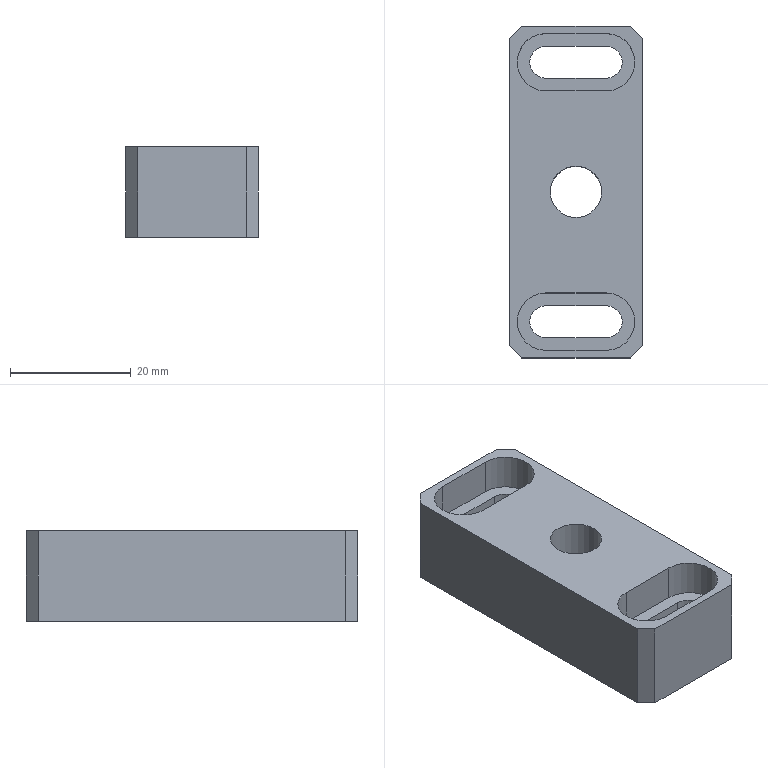Part | NX | 1 solid | 29 faces | box 22 x 55 x 15 mm | volume 13837 mm3 | plane 20 | cylinder 9 | commonest cylinder face diameters 5.3 x4 9.5 x4 8.5 x1
STEP:
#1=CARTESIAN_POINT('',(-5.,16.75,15.));
#2=VERTEX_POINT('',#1);
#3=CARTESIAN_POINT('',(5.,16.75,15.));
#4=VERTEX_POINT('',#3);
#5=CARTESIAN_POINT('',(-5.,16.75,15.));
#6=DIRECTION('',(1.,0.,0.));
#7=VECTOR('',#6,1000.);
#8=LINE('',#5,#7);
#9=EDGE_CURVE('',#2,#4,#8,.T.);
#10=ORIENTED_EDGE('',*,*,#9,.F.);
#11=CARTESIAN_POINT('',(-5.,26.25,15.));
#12=VERTEX_POINT('',#11);
#13=CARTESIAN_POINT('',(-5.,21.5,15.));
#14=DIRECTION('',(0.,0.,1.));
#15=DIRECTION('',(1.,0.,0.));
#16=AXIS2_PLACEMENT_3D('',#13,#14,#15);
#17=CIRCLE('',#16,4.75);
#18=EDGE_CURVE('',#12,#2,#17,.T.);
#19=ORIENTED_EDGE('',*,*,#18,.F.);
#20=CARTESIAN_POINT('',(5.,26.25,15.));
#21=VERTEX_POINT('',#20);
#22=CARTESIAN_POINT('',(-5.,26.25,15.));
#23=DIRECTION('',(-1.,0.,0.));
#24=VECTOR('',#23,1000.);
#25=LINE('',#22,#24);
#26=EDGE_CURVE('',#21,#12,#25,.T.);
#27=ORIENTED_EDGE('',*,*,#26,.F.);
#28=CARTESIAN_POINT('',(5.,21.5,15.));
#29=DIRECTION('',(0.,0.,1.));
#30=DIRECTION('',(1.,0.,0.));
#31=AXIS2_PLACEMENT_3D('',#28,#29,#30);
#32=CIRCLE('',#31,4.75);
#33=EDGE_CURVE('',#4,#21,#32,.T.);
#34=ORIENTED_EDGE('',*,*,#33,.F.);
#35=EDGE_LOOP('',(#10,#19,#27,#34));
#36=FACE_BOUND('',#35,.T.);
#37=CARTESIAN_POINT('',(4.25,0.,15.));
#38=VERTEX_POINT('',#37);
#39=CARTESIAN_POINT('',(0.,0.,15.));
#40=DIRECTION('',(0.,0.,1.));
#41=DIRECTION('',(1.,0.,0.));
#42=AXIS2_PLACEMENT_3D('',#39,#40,#41);
#43=CIRCLE('',#42,4.25);
#44=EDGE_CURVE('',#38,#38,#43,.T.);
#45=ORIENTED_EDGE('',*,*,#44,.F.);
#46=EDGE_LOOP('',(#45));
#47=FACE_BOUND('',#46,.T.);
#48=CARTESIAN_POINT('',(-11.,25.5,15.));
#49=VERTEX_POINT('',#48);
#50=CARTESIAN_POINT('',(-11.,-25.5,15.));
#51=VERTEX_POINT('',#50);
#52=CARTESIAN_POINT('',(-11.,-27.5,15.));
#53=DIRECTION('',(0.,-1.,0.));
#54=VECTOR('',#53,1000.);
#55=LINE('',#52,#54);
#56=EDGE_CURVE('',#49,#51,#55,.T.);
#57=ORIENTED_EDGE('',*,*,#56,.T.);
#58=CARTESIAN_POINT('',(-9.,-27.5,15.));
#59=VERTEX_POINT('',#58);
#60=CARTESIAN_POINT('',(-9.,-27.5,15.));
#61=DIRECTION('',(-0.7071,0.7071,0.));
#62=VECTOR('',#61,1000.);
#63=LINE('',#60,#62);
#64=EDGE_CURVE('',#51,#59,#63,.F.);
#65=ORIENTED_EDGE('',*,*,#64,.T.);
#66=CARTESIAN_POINT('',(9.,-27.5,15.));
#67=VERTEX_POINT('',#66);
#68=CARTESIAN_POINT('',(-11.,-27.5,15.));
#69=DIRECTION('',(1.,0.,0.));
#70=VECTOR('',#69,1000.);
#71=LINE('',#68,#70);
#72=EDGE_CURVE('',#59,#67,#71,.T.);
#73=ORIENTED_EDGE('',*,*,#72,.T.);
#74=CARTESIAN_POINT('',(11.,-25.5,15.));
#75=VERTEX_POINT('',#74);
#76=CARTESIAN_POINT('',(11.,-25.5,15.));
#77=DIRECTION('',(-0.7071,-0.7071,0.));
#78=VECTOR('',#77,1000.);
#79=LINE('',#76,#78);
#80=EDGE_CURVE('',#67,#75,#79,.F.);
#81=ORIENTED_EDGE('',*,*,#80,.T.);
#82=CARTESIAN_POINT('',(11.,25.5,15.));
#83=VERTEX_POINT('',#82);
#84=CARTESIAN_POINT('',(11.,-27.5,15.));
#85=DIRECTION('',(0.,1.,0.));
#86=VECTOR('',#85,1000.);
#87=LINE('',#84,#86);
#88=EDGE_CURVE('',#75,#83,#87,.T.);
#89=ORIENTED_EDGE('',*,*,#88,.T.);
#90=CARTESIAN_POINT('',(9.,27.5,15.));
#91=VERTEX_POINT('',#90);
#92=CARTESIAN_POINT('',(9.,27.5,15.));
#93=DIRECTION('',(0.7071,-0.7071,0.));
#94=VECTOR('',#93,1000.);
#95=LINE('',#92,#94);
#96=EDGE_CURVE('',#83,#91,#95,.F.);
#97=ORIENTED_EDGE('',*,*,#96,.T.);
#98=CARTESIAN_POINT('',(-9.,27.5,15.));
#99=VERTEX_POINT('',#98);
#100=CARTESIAN_POINT('',(-11.,27.5,15.));
#101=DIRECTION('',(-1.,0.,0.));
#102=VECTOR('',#101,1000.);
#103=LINE('',#100,#102);
#104=EDGE_CURVE('',#91,#99,#103,.T.);
#105=ORIENTED_EDGE('',*,*,#104,.T.);
#106=CARTESIAN_POINT('',(-11.,25.5,15.));
#107=DIRECTION('',(0.7071,0.7071,0.));
#108=VECTOR('',#107,1000.);
#109=LINE('',#106,#108);
#110=EDGE_CURVE('',#99,#49,#109,.F.);
#111=ORIENTED_EDGE('',*,*,#110,.T.);
#112=EDGE_LOOP('',(#57,#65,#73,#81,#89,#97,#105,#111));
#113=FACE_BOUND('',#112,.T.);
#114=CARTESIAN_POINT('',(-5.,-26.25,15.));
#115=VERTEX_POINT('',#114);
#116=CARTESIAN_POINT('',(-5.,-16.75,15.));
#117=VERTEX_POINT('',#116);
#118=CARTESIAN_POINT('',(-5.,-21.5,15.));
#119=DIRECTION('',(0.,0.,-1.));
#120=DIRECTION('',(1.,0.,0.));
#121=AXIS2_PLACEMENT_3D('',#118,#119,#120);
#122=CIRCLE('',#121,4.75);
#123=EDGE_CURVE('',#115,#117,#122,.T.);
#124=ORIENTED_EDGE('',*,*,#123,.T.);
#125=CARTESIAN_POINT('',(5.,-16.75,15.));
#126=VERTEX_POINT('',#125);
#127=CARTESIAN_POINT('',(-5.,-16.75,15.));
#128=DIRECTION('',(1.,0.,0.));
#129=VECTOR('',#128,1000.);
#130=LINE('',#127,#129);
#131=EDGE_CURVE('',#117,#126,#130,.T.);
#132=ORIENTED_EDGE('',*,*,#131,.T.);
#133=CARTESIAN_POINT('',(5.,-26.25,15.));
#134=VERTEX_POINT('',#133);
#135=CARTESIAN_POINT('',(5.,-21.5,15.));
#136=DIRECTION('',(0.,0.,-1.));
#137=DIRECTION('',(1.,0.,0.));
#138=AXIS2_PLACEMENT_3D('',#135,#136,#137);
#139=CIRCLE('',#138,4.75);
#140=EDGE_CURVE('',#126,#134,#139,.T.);
#141=ORIENTED_EDGE('',*,*,#140,.T.);
#142=CARTESIAN_POINT('',(-5.,-26.25,15.));
#143=DIRECTION('',(-1.,0.,0.));
#144=VECTOR('',#143,1000.);
#145=LINE('',#142,#144);
#146=EDGE_CURVE('',#134,#115,#145,.T.);
#147=ORIENTED_EDGE('',*,*,#146,.T.);
#148=EDGE_LOOP('',(#124,#132,#141,#147));
#149=FACE_BOUND('',#148,.T.);
#150=CARTESIAN_POINT('',(0.,0.,15.));
#151=DIRECTION('',(0.,0.,-1.));
#152=DIRECTION('',(-1.,0.,0.));
#153=AXIS2_PLACEMENT_3D('',#150,#151,#152);
#154=PLANE('',#153);
#155=ADVANCED_FACE('',(#36,#47,#113,#149),#154,.F.);
#156=CARTESIAN_POINT('',(-5.,-18.85,0.));
#157=VERTEX_POINT('',#156);
#158=CARTESIAN_POINT('',(-5.,-18.85,9.));
#159=VERTEX_POINT('',#158);
#160=CARTESIAN_POINT('',(-5.,-18.85,0.));
#161=DIRECTION('',(0.,0.,1.));
#162=VECTOR('',#161,1000.);
#163=LINE('',#160,#162);
#164=EDGE_CURVE('',#157,#159,#163,.T.);
#165=ORIENTED_EDGE('',*,*,#164,.T.);
#166=CARTESIAN_POINT('',(-5.,-24.15,9.));
#167=VERTEX_POINT('',#166);
#168=CARTESIAN_POINT('',(-5.,-21.5,9.));
#169=DIRECTION('',(0.,0.,1.));
#170=DIRECTION('',(1.,0.,0.));
#171=AXIS2_PLACEMENT_3D('',#168,#169,#170);
#172=CIRCLE('',#171,2.65);
#173=EDGE_CURVE('',#159,#167,#172,.T.);
#174=ORIENTED_EDGE('',*,*,#173,.T.);
#175=CARTESIAN_POINT('',(-5.,-24.15,0.));
#176=VERTEX_POINT('',#175);
#177=CARTESIAN_POINT('',(-5.,-24.15,0.));
#178=DIRECTION('',(0.,0.,1.));
#179=VECTOR('',#178,1000.);
#180=LINE('',#177,#179);
#181=EDGE_CURVE('',#176,#167,#180,.T.);
#182=ORIENTED_EDGE('',*,*,#181,.F.);
#183=CARTESIAN_POINT('',(-5.,-21.5,0.));
#184=DIRECTION('',(0.,0.,-1.));
#185=DIRECTION('',(1.,0.,0.));
#186=AXIS2_PLACEMENT_3D('',#183,#184,#185);
#187=CIRCLE('',#186,2.65);
#188=EDGE_CURVE('',#176,#157,#187,.T.);
#189=ORIENTED_EDGE('',*,*,#188,.T.);
#190=EDGE_LOOP('',(#165,#174,#182,#189));
#191=FACE_BOUND('',#190,.T.);
#192=CARTESIAN_POINT('',(-5.,-21.5,0.));
#193=DIRECTION('',(0.,0.,1.));
#194=DIRECTION('',(1.,0.,0.));
#195=AXIS2_PLACEMENT_3D('',#192,#193,#194);
#196=CYLINDRICAL_SURFACE('',#195,2.65);
#197=ADVANCED_FACE('',(#191),#196,.F.);
#198=CARTESIAN_POINT('',(5.,-18.85,0.));
#199=VERTEX_POINT('',#198);
#200=CARTESIAN_POINT('',(5.,-18.85,9.));
#201=VERTEX_POINT('',#200);
#202=CARTESIAN_POINT('',(5.,-18.85,0.));
#203=DIRECTION('',(0.,0.,1.));
#204=VECTOR('',#203,1000.);
#205=LINE('',#202,#204);
#206=EDGE_CURVE('',#199,#201,#205,.T.);
#207=ORIENTED_EDGE('',*,*,#206,.T.);
#208=CARTESIAN_POINT('',(-5.,-18.85,9.));
#209=DIRECTION('',(-1.,0.,0.));
#210=VECTOR('',#209,1000.);
#211=LINE('',#208,#210);
#212=EDGE_CURVE('',#201,#159,#211,.T.);
#213=ORIENTED_EDGE('',*,*,#212,.T.);
#214=ORIENTED_EDGE('',*,*,#164,.F.);
#215=CARTESIAN_POINT('',(-5.,-18.85,0.));
#216=DIRECTION('',(1.,0.,0.));
#217=VECTOR('',#216,1000.);
#218=LINE('',#215,#217);
#219=EDGE_CURVE('',#157,#199,#218,.T.);
#220=ORIENTED_EDGE('',*,*,#219,.T.);
#221=EDGE_LOOP('',(#207,#213,#214,#220));
#222=FACE_BOUND('',#221,.T.);
#223=CARTESIAN_POINT('',(-5.,-18.85,0.));
#224=DIRECTION('',(0.,-1.,0.));
#225=DIRECTION('',(0.,0.,-1.));
#226=AXIS2_PLACEMENT_3D('',#223,#224,#225);
#227=PLANE('',#226);
#228=ADVANCED_FACE('',(#222),#227,.T.);
#229=CARTESIAN_POINT('',(5.,-24.15,0.));
#230=VERTEX_POINT('',#229);
#231=CARTESIAN_POINT('',(5.,-24.15,9.));
#232=VERTEX_POINT('',#231);
#233=CARTESIAN_POINT('',(5.,-24.15,0.));
#234=DIRECTION('',(0.,0.,1.));
#235=VECTOR('',#234,1000.);
#236=LINE('',#233,#235);
#237=EDGE_CURVE('',#230,#232,#236,.T.);
#238=ORIENTED_EDGE('',*,*,#237,.T.);
#239=CARTESIAN_POINT('',(5.,-21.5,9.));
#240=DIRECTION('',(0.,0.,1.));
#241=DIRECTION('',(1.,0.,0.));
#242=AXIS2_PLACEMENT_3D('',#239,#240,#241);
#243=CIRCLE('',#242,2.65);
#244=EDGE_CURVE('',#232,#201,#243,.T.);
#245=ORIENTED_EDGE('',*,*,#244,.T.);
#246=ORIENTED_EDGE('',*,*,#206,.F.);
#247=CARTESIAN_POINT('',(5.,-21.5,0.));
#248=DIRECTION('',(0.,0.,-1.));
#249=DIRECTION('',(1.,0.,0.));
#250=AXIS2_PLACEMENT_3D('',#247,#248,#249);
#251=CIRCLE('',#250,2.65);
#252=EDGE_CURVE('',#199,#230,#251,.T.);
#253=ORIENTED_EDGE('',*,*,#252,.T.);
#254=EDGE_LOOP('',(#238,#245,#246,#253));
#255=FACE_BOUND('',#254,.T.);
#256=CARTESIAN_POINT('',(5.,-21.5,0.));
#257=DIRECTION('',(0.,0.,1.));
#258=DIRECTION('',(1.,0.,0.));
#259=AXIS2_PLACEMENT_3D('',#256,#257,#258);
#260=CYLINDRICAL_SURFACE('',#259,2.65);
#261=ADVANCED_FACE('',(#255),#260,.F.);
#262=ORIENTED_EDGE('',*,*,#181,.T.);
#263=CARTESIAN_POINT('',(-5.,-24.15,9.));
#264=DIRECTION('',(1.,0.,0.));
#265=VECTOR('',#264,1000.);
#266=LINE('',#263,#265);
#267=EDGE_CURVE('',#167,#232,#266,.T.);
#268=ORIENTED_EDGE('',*,*,#267,.T.);
#269=ORIENTED_EDGE('',*,*,#237,.F.);
#270=CARTESIAN_POINT('',(-5.,-24.15,0.));
#271=DIRECTION('',(-1.,0.,0.));
#272=VECTOR('',#271,1000.);
#273=LINE('',#270,#272);
#274=EDGE_CURVE('',#230,#176,#273,.T.);
#275=ORIENTED_EDGE('',*,*,#274,.T.);
#276=EDGE_LOOP('',(#262,#268,#269,#275));
#277=FACE_BOUND('',#276,.T.);
#278=CARTESIAN_POINT('',(-5.,-24.15,0.));
#279=DIRECTION('',(0.,1.,0.));
#280=DIRECTION('',(0.,0.,1.));
#281=AXIS2_PLACEMENT_3D('',#278,#279,#280);
#282=PLANE('',#281);
#283=ADVANCED_FACE('',(#277),#282,.T.);
#284=CARTESIAN_POINT('',(-9.,-27.5,0.));
#285=VERTEX_POINT('',#284);
#286=CARTESIAN_POINT('',(9.,-27.5,0.));
#287=VERTEX_POINT('',#286);
#288=CARTESIAN_POINT('',(-11.,-27.5,0.));
#289=DIRECTION('',(1.,0.,0.));
#290=VECTOR('',#289,1000.);
#291=LINE('',#288,#290);
#292=EDGE_CURVE('',#285,#287,#291,.T.);
#293=ORIENTED_EDGE('',*,*,#292,.F.);
#294=CARTESIAN_POINT('',(-11.,-25.5,0.));
#295=VERTEX_POINT('',#294);
#296=CARTESIAN_POINT('',(-18.25,-18.25,0.));
#297=DIRECTION('',(0.7071,-0.7071,0.));
#298=VECTOR('',#297,1000.);
#299=LINE('',#296,#298);
#300=EDGE_CURVE('',#285,#295,#299,.F.);
#301=ORIENTED_EDGE('',*,*,#300,.T.);
#302=CARTESIAN_POINT('',(-11.,25.5,0.));
#303=VERTEX_POINT('',#302);
#304=CARTESIAN_POINT('',(-11.,-27.5,0.));
#305=DIRECTION('',(0.,-1.,0.));
#306=VECTOR('',#305,1000.);
#307=LINE('',#304,#306);
#308=EDGE_CURVE('',#303,#295,#307,.T.);
#309=ORIENTED_EDGE('',*,*,#308,.F.);
#310=CARTESIAN_POINT('',(-9.,27.5,0.));
#311=VERTEX_POINT('',#310);
#312=CARTESIAN_POINT('',(-18.25,18.25,0.));
#313=DIRECTION('',(-0.7071,-0.7071,0.));
#314=VECTOR('',#313,1000.);
#315=LINE('',#312,#314);
#316=EDGE_CURVE('',#303,#311,#315,.F.);
#317=ORIENTED_EDGE('',*,*,#316,.T.);
#318=CARTESIAN_POINT('',(9.,27.5,0.));
#319=VERTEX_POINT('',#318);
#320=CARTESIAN_POINT('',(-11.,27.5,0.));
#321=DIRECTION('',(-1.,0.,0.));
#322=VECTOR('',#321,1000.);
#323=LINE('',#320,#322);
#324=EDGE_CURVE('',#319,#311,#323,.T.);
#325=ORIENTED_EDGE('',*,*,#324,.F.);
#326=CARTESIAN_POINT('',(11.,25.5,0.));
#327=VERTEX_POINT('',#326);
#328=CARTESIAN_POINT('',(18.25,18.25,0.));
#329=DIRECTION('',(-0.7071,0.7071,0.));
#330=VECTOR('',#329,1000.);
#331=LINE('',#328,#330);
#332=EDGE_CURVE('',#319,#327,#331,.F.);
#333=ORIENTED_EDGE('',*,*,#332,.T.);
#334=CARTESIAN_POINT('',(11.,-25.5,0.));
#335=VERTEX_POINT('',#334);
#336=CARTESIAN_POINT('',(11.,-27.5,0.));
#337=DIRECTION('',(0.,1.,0.));
#338=VECTOR('',#337,1000.);
#339=LINE('',#336,#338);
#340=EDGE_CURVE('',#335,#327,#339,.T.);
#341=ORIENTED_EDGE('',*,*,#340,.F.);
#342=CARTESIAN_POINT('',(18.25,-18.25,0.));
#343=DIRECTION('',(0.7071,0.7071,0.));
#344=VECTOR('',#343,1000.);
#345=LINE('',#342,#344);
#346=EDGE_CURVE('',#335,#287,#345,.F.);
#347=ORIENTED_EDGE('',*,*,#346,.T.);
#348=EDGE_LOOP('',(#293,#301,#309,#317,#325,#333,#341,#347));
#349=FACE_BOUND('',#348,.T.);
#350=CARTESIAN_POINT('',(4.25,0.,0.));
#351=VERTEX_POINT('',#350);
#352=CARTESIAN_POINT('',(0.,0.,0.));
#353=DIRECTION('',(0.,0.,1.));
#354=DIRECTION('',(1.,0.,0.));
#355=AXIS2_PLACEMENT_3D('',#352,#353,#354);
#356=CIRCLE('',#355,4.25);
#357=EDGE_CURVE('',#351,#351,#356,.T.);
#358=ORIENTED_EDGE('',*,*,#357,.T.);
#359=EDGE_LOOP('',(#358));
#360=FACE_BOUND('',#359,.T.);
#361=CARTESIAN_POINT('',(-5.,24.15,0.));
#362=VERTEX_POINT('',#361);
#363=CARTESIAN_POINT('',(-5.,18.85,0.));
#364=VERTEX_POINT('',#363);
#365=CARTESIAN_POINT('',(-5.,21.5,0.));
#366=DIRECTION('',(0.,0.,1.));
#367=DIRECTION('',(1.,0.,0.));
#368=AXIS2_PLACEMENT_3D('',#365,#366,#367);
#369=CIRCLE('',#368,2.65);
#370=EDGE_CURVE('',#362,#364,#369,.T.);
#371=ORIENTED_EDGE('',*,*,#370,.T.);
#372=CARTESIAN_POINT('',(5.,18.85,0.));
#373=VERTEX_POINT('',#372);
#374=CARTESIAN_POINT('',(-5.,18.85,0.));
#375=DIRECTION('',(1.,0.,0.));
#376=VECTOR('',#375,1000.);
#377=LINE('',#374,#376);
#378=EDGE_CURVE('',#364,#373,#377,.T.);
#379=ORIENTED_EDGE('',*,*,#378,.T.);
#380=CARTESIAN_POINT('',(5.,24.15,0.));
#381=VERTEX_POINT('',#380);
#382=CARTESIAN_POINT('',(5.,21.5,0.));
#383=DIRECTION('',(0.,0.,1.));
#384=DIRECTION('',(1.,0.,0.));
#385=AXIS2_PLACEMENT_3D('',#382,#383,#384);
#386=CIRCLE('',#385,2.65);
#387=EDGE_CURVE('',#373,#381,#386,.T.);
#388=ORIENTED_EDGE('',*,*,#387,.T.);
#389=CARTESIAN_POINT('',(-5.,24.15,0.));
#390=DIRECTION('',(-1.,0.,0.));
#391=VECTOR('',#390,1000.);
#392=LINE('',#389,#391);
#393=EDGE_CURVE('',#381,#362,#392,.T.);
#394=ORIENTED_EDGE('',*,*,#393,.T.);
#395=EDGE_LOOP('',(#371,#379,#388,#394));
#396=FACE_BOUND('',#395,.T.);
#397=ORIENTED_EDGE('',*,*,#219,.F.);
#398=ORIENTED_EDGE('',*,*,#188,.F.);
#399=ORIENTED_EDGE('',*,*,#274,.F.);
#400=ORIENTED_EDGE('',*,*,#252,.F.);
#401=EDGE_LOOP('',(#397,#398,#399,#400));
#402=FACE_BOUND('',#401,.T.);
#403=CARTESIAN_POINT('',(0.,0.,0.));
#404=DIRECTION('',(0.,0.,-1.));
#405=DIRECTION('',(-1.,0.,0.));
#406=AXIS2_PLACEMENT_3D('',#403,#404,#405);
#407=PLANE('',#406);
#408=ADVANCED_FACE('',(#349,#360,#396,#402),#407,.T.);
#409=CARTESIAN_POINT('',(-5.,18.85,9.));
#410=VERTEX_POINT('',#409);
#411=CARTESIAN_POINT('',(-5.,24.15,9.));
#412=VERTEX_POINT('',#411);
#413=CARTESIAN_POINT('',(-5.,21.5,9.));
#414=DIRECTION('',(0.,0.,1.));
#415=DIRECTION('',(1.,0.,0.));
#416=AXIS2_PLACEMENT_3D('',#413,#414,#415);
#417=CIRCLE('',#416,2.65);
#418=EDGE_CURVE('',#410,#412,#417,.F.);
#419=ORIENTED_EDGE('',*,*,#418,.F.);
#420=CARTESIAN_POINT('',(-5.,18.85,0.));
#421=DIRECTION('',(0.,0.,1.));
#422=VECTOR('',#421,1000.);
#423=LINE('',#420,#422);
#424=EDGE_CURVE('',#364,#410,#423,.T.);
#425=ORIENTED_EDGE('',*,*,#424,.F.);
#426=ORIENTED_EDGE('',*,*,#370,.F.);
#427=CARTESIAN_POINT('',(-5.,24.15,0.));
#428=DIRECTION('',(0.,0.,1.));
#429=VECTOR('',#428,1000.);
#430=LINE('',#427,#429);
#431=EDGE_CURVE('',#362,#412,#430,.T.);
#432=ORIENTED_EDGE('',*,*,#431,.T.);
#433=EDGE_LOOP('',(#419,#425,#426,#432));
#434=FACE_BOUND('',#433,.T.);
#435=CARTESIAN_POINT('',(-5.,21.5,0.));
#436=DIRECTION('',(0.,0.,1.));
#437=DIRECTION('',(1.,0.,0.));
#438=AXIS2_PLACEMENT_3D('',#435,#436,#437);
#439=CYLINDRICAL_SURFACE('',#438,2.65);
#440=ADVANCED_FACE('',(#434),#439,.F.);
#441=CARTESIAN_POINT('',(5.,24.15,9.));
#442=VERTEX_POINT('',#441);
#443=CARTESIAN_POINT('',(-5.,24.15,9.));
#444=DIRECTION('',(1.,0.,0.));
#445=VECTOR('',#444,1000.);
#446=LINE('',#443,#445);
#447=EDGE_CURVE('',#412,#442,#446,.T.);
#448=ORIENTED_EDGE('',*,*,#447,.F.);
#449=ORIENTED_EDGE('',*,*,#431,.F.);
#450=ORIENTED_EDGE('',*,*,#393,.F.);
#451=CARTESIAN_POINT('',(5.,24.15,0.));
#452=DIRECTION('',(0.,0.,1.));
#453=VECTOR('',#452,1000.);
#454=LINE('',#451,#453);
#455=EDGE_CURVE('',#381,#442,#454,.T.);
#456=ORIENTED_EDGE('',*,*,#455,.T.);
#457=EDGE_LOOP('',(#448,#449,#450,#456));
#458=FACE_BOUND('',#457,.T.);
#459=CARTESIAN_POINT('',(-5.,24.15,0.));
#460=DIRECTION('',(0.,1.,0.));
#461=DIRECTION('',(0.,0.,1.));
#462=AXIS2_PLACEMENT_3D('',#459,#460,#461);
#463=PLANE('',#462);
#464=ADVANCED_FACE('',(#458),#463,.F.);
#465=CARTESIAN_POINT('',(5.,18.85,9.));
#466=VERTEX_POINT('',#465);
#467=CARTESIAN_POINT('',(5.,21.5,9.));
#468=DIRECTION('',(0.,0.,1.));
#469=DIRECTION('',(1.,0.,0.));
#470=AXIS2_PLACEMENT_3D('',#467,#468,#469);
#471=CIRCLE('',#470,2.65);
#472=EDGE_CURVE('',#442,#466,#471,.F.);
#473=ORIENTED_EDGE('',*,*,#472,.F.);
#474=ORIENTED_EDGE('',*,*,#455,.F.);
#475=ORIENTED_EDGE('',*,*,#387,.F.);
#476=CARTESIAN_POINT('',(5.,18.85,0.));
#477=DIRECTION('',(0.,0.,1.));
#478=VECTOR('',#477,1000.);
#479=LINE('',#476,#478);
#480=EDGE_CURVE('',#373,#466,#479,.T.);
#481=ORIENTED_EDGE('',*,*,#480,.T.);
#482=EDGE_LOOP('',(#473,#474,#475,#481));
#483=FACE_BOUND('',#482,.T.);
#484=CARTESIAN_POINT('',(5.,21.5,0.));
#485=DIRECTION('',(0.,0.,1.));
#486=DIRECTION('',(1.,0.,0.));
#487=AXIS2_PLACEMENT_3D('',#484,#485,#486);
#488=CYLINDRICAL_SURFACE('',#487,2.65);
#489=ADVANCED_FACE('',(#483),#488,.F.);
#490=CARTESIAN_POINT('',(-5.,18.85,9.));
#491=DIRECTION('',(-1.,0.,0.));
#492=VECTOR('',#491,1000.);
#493=LINE('',#490,#492);
#494=EDGE_CURVE('',#466,#410,#493,.T.);
#495=ORIENTED_EDGE('',*,*,#494,.F.);
#496=ORIENTED_EDGE('',*,*,#480,.F.);
#497=ORIENTED_EDGE('',*,*,#378,.F.);
#498=ORIENTED_EDGE('',*,*,#424,.T.);
#499=EDGE_LOOP('',(#495,#496,#497,#498));
#500=FACE_BOUND('',#499,.T.);
#501=CARTESIAN_POINT('',(-5.,18.85,0.));
#502=DIRECTION('',(0.,-1.,0.));
#503=DIRECTION('',(0.,0.,-1.));
#504=AXIS2_PLACEMENT_3D('',#501,#502,#503);
#505=PLANE('',#504);
#506=ADVANCED_FACE('',(#500),#505,.F.);
#507=ORIENTED_EDGE('',*,*,#88,.F.);
#508=CARTESIAN_POINT('',(11.,-25.5,15.));
#509=DIRECTION('',(0.,0.,-1.));
#510=VECTOR('',#509,1000.);
#511=LINE('',#508,#510);
#512=EDGE_CURVE('',#75,#335,#511,.T.);
#513=ORIENTED_EDGE('',*,*,#512,.T.);
#514=ORIENTED_EDGE('',*,*,#340,.T.);
#515=CARTESIAN_POINT('',(11.,25.5,15.));
#516=DIRECTION('',(0.,0.,1.));
#517=VECTOR('',#516,1000.);
#518=LINE('',#515,#517);
#519=EDGE_CURVE('',#327,#83,#518,.T.);
#520=ORIENTED_EDGE('',*,*,#519,.T.);
#521=EDGE_LOOP('',(#507,#513,#514,#520));
#522=FACE_BOUND('',#521,.T.);
#523=CARTESIAN_POINT('',(11.,-27.5,15.));
#524=DIRECTION('',(-1.,0.,0.));
#525=DIRECTION('',(0.,0.,1.));
#526=AXIS2_PLACEMENT_3D('',#523,#524,#525);
#527=PLANE('',#526);
#528=ADVANCED_FACE('',(#522),#527,.F.);
#529=ORIENTED_EDGE('',*,*,#324,.T.);
#530=CARTESIAN_POINT('',(-9.,27.5,15.));
#531=DIRECTION('',(0.,0.,1.));
#532=VECTOR('',#531,1000.);
#533=LINE('',#530,#532);
#534=EDGE_CURVE('',#311,#99,#533,.T.);
#535=ORIENTED_EDGE('',*,*,#534,.T.);
#536=ORIENTED_EDGE('',*,*,#104,.F.);
#537=CARTESIAN_POINT('',(9.,27.5,15.));
#538=DIRECTION('',(0.,0.,-1.));
#539=VECTOR('',#538,1000.);
#540=LINE('',#537,#539);
#541=EDGE_CURVE('',#91,#319,#540,.T.);
#542=ORIENTED_EDGE('',*,*,#541,.T.);
#543=EDGE_LOOP('',(#529,#535,#536,#542));
#544=FACE_BOUND('',#543,.T.);
#545=CARTESIAN_POINT('',(-11.,27.5,15.));
#546=DIRECTION('',(0.,-1.,0.));
#547=DIRECTION('',(0.,0.,-1.));
#548=AXIS2_PLACEMENT_3D('',#545,#546,#547);
#549=PLANE('',#548);
#550=ADVANCED_FACE('',(#544),#549,.F.);
#551=ORIENTED_EDGE('',*,*,#308,.T.);
#552=CARTESIAN_POINT('',(-11.,-25.5,15.));
#553=DIRECTION('',(0.,0.,1.));
#554=VECTOR('',#553,1000.);
#555=LINE('',#552,#554);
#556=EDGE_CURVE('',#295,#51,#555,.T.);
#557=ORIENTED_EDGE('',*,*,#556,.T.);
#558=ORIENTED_EDGE('',*,*,#56,.F.);
#559=CARTESIAN_POINT('',(-11.,25.5,15.));
#560=DIRECTION('',(0.,0.,-1.));
#561=VECTOR('',#560,1000.);
#562=LINE('',#559,#561);
#563=EDGE_CURVE('',#49,#303,#562,.T.);
#564=ORIENTED_EDGE('',*,*,#563,.T.);
#565=EDGE_LOOP('',(#551,#557,#558,#564));
#566=FACE_BOUND('',#565,.T.);
#567=CARTESIAN_POINT('',(-11.,-27.5,15.));
#568=DIRECTION('',(1.,0.,0.));
#569=DIRECTION('',(0.,0.,-1.));
#570=AXIS2_PLACEMENT_3D('',#567,#568,#569);
#571=PLANE('',#570);
#572=ADVANCED_FACE('',(#566),#571,.F.);
#573=ORIENTED_EDGE('',*,*,#72,.F.);
#574=CARTESIAN_POINT('',(-9.,-27.5,15.));
#575=DIRECTION('',(0.,0.,-1.));
#576=VECTOR('',#575,1000.);
#577=LINE('',#574,#576);
#578=EDGE_CURVE('',#59,#285,#577,.T.);
#579=ORIENTED_EDGE('',*,*,#578,.T.);
#580=ORIENTED_EDGE('',*,*,#292,.T.);
#581=CARTESIAN_POINT('',(9.,-27.5,15.));
#582=DIRECTION('',(0.,0.,1.));
#583=VECTOR('',#582,1000.);
#584=LINE('',#581,#583);
#585=EDGE_CURVE('',#287,#67,#584,.T.);
#586=ORIENTED_EDGE('',*,*,#585,.T.);
#587=EDGE_LOOP('',(#573,#579,#580,#586));
#588=FACE_BOUND('',#587,.T.);
#589=CARTESIAN_POINT('',(-11.,-27.5,15.));
#590=DIRECTION('',(0.,1.,0.));
#591=DIRECTION('',(0.,0.,1.));
#592=AXIS2_PLACEMENT_3D('',#589,#590,#591);
#593=PLANE('',#592);
#594=ADVANCED_FACE('',(#588),#593,.F.);
#595=ORIENTED_EDGE('',*,*,#357,.F.);
#596=EDGE_LOOP('',(#595));
#597=FACE_BOUND('',#596,.T.);
#598=ORIENTED_EDGE('',*,*,#44,.T.);
#599=EDGE_LOOP('',(#598));
#600=FACE_BOUND('',#599,.T.);
#601=CARTESIAN_POINT('',(0.,0.,15.));
#602=DIRECTION('',(0.,0.,1.));
#603=DIRECTION('',(1.,0.,0.));
#604=AXIS2_PLACEMENT_3D('',#601,#602,#603);
#605=CYLINDRICAL_SURFACE('',#604,4.25);
#606=ADVANCED_FACE('',(#597,#600),#605,.F.);
#607=CARTESIAN_POINT('',(-5.,26.25,9.));
#608=VERTEX_POINT('',#607);
#609=CARTESIAN_POINT('',(-5.,16.75,9.));
#610=VERTEX_POINT('',#609);
#611=CARTESIAN_POINT('',(-5.,21.5,9.));
#612=DIRECTION('',(0.,0.,1.));
#613=DIRECTION('',(1.,0.,0.));
#614=AXIS2_PLACEMENT_3D('',#611,#612,#613);
#615=CIRCLE('',#614,4.75);
#616=EDGE_CURVE('',#608,#610,#615,.T.);
#617=ORIENTED_EDGE('',*,*,#616,.T.);
#618=CARTESIAN_POINT('',(5.,16.75,9.));
#619=VERTEX_POINT('',#618);
#620=CARTESIAN_POINT('',(-5.,16.75,9.));
#621=DIRECTION('',(1.,0.,0.));
#622=VECTOR('',#621,1000.);
#623=LINE('',#620,#622);
#624=EDGE_CURVE('',#610,#619,#623,.T.);
#625=ORIENTED_EDGE('',*,*,#624,.T.);
#626=CARTESIAN_POINT('',(5.,26.25,9.));
#627=VERTEX_POINT('',#626);
#628=CARTESIAN_POINT('',(5.,21.5,9.));
#629=DIRECTION('',(0.,0.,1.));
#630=DIRECTION('',(1.,0.,0.));
#631=AXIS2_PLACEMENT_3D('',#628,#629,#630);
#632=CIRCLE('',#631,4.75);
#633=EDGE_CURVE('',#619,#627,#632,.T.);
#634=ORIENTED_EDGE('',*,*,#633,.T.);
#635=CARTESIAN_POINT('',(-5.,26.25,9.));
#636=DIRECTION('',(-1.,0.,0.));
#637=VECTOR('',#636,1000.);
#638=LINE('',#635,#637);
#639=EDGE_CURVE('',#627,#608,#638,.T.);
#640=ORIENTED_EDGE('',*,*,#639,.T.);
#641=EDGE_LOOP('',(#617,#625,#634,#640));
#642=FACE_BOUND('',#641,.T.);
#643=ORIENTED_EDGE('',*,*,#418,.T.);
#644=ORIENTED_EDGE('',*,*,#447,.T.);
#645=ORIENTED_EDGE('',*,*,#472,.T.);
#646=ORIENTED_EDGE('',*,*,#494,.T.);
#647=EDGE_LOOP('',(#643,#644,#645,#646));
#648=FACE_BOUND('',#647,.T.);
#649=CARTESIAN_POINT('',(-5.,21.5,9.));
#650=DIRECTION('',(0.,0.,1.));
#651=DIRECTION('',(1.,0.,0.));
#652=AXIS2_PLACEMENT_3D('',#649,#650,#651);
#653=PLANE('',#652);
#654=ADVANCED_FACE('',(#642,#648),#653,.T.);
#655=ORIENTED_EDGE('',*,*,#18,.T.);
#656=CARTESIAN_POINT('',(-5.,16.75,9.));
#657=DIRECTION('',(0.,0.,1.));
#658=VECTOR('',#657,1000.);
#659=LINE('',#656,#658);
#660=EDGE_CURVE('',#610,#2,#659,.T.);
#661=ORIENTED_EDGE('',*,*,#660,.F.);
#662=ORIENTED_EDGE('',*,*,#616,.F.);
#663=CARTESIAN_POINT('',(-5.,26.25,9.));
#664=DIRECTION('',(0.,0.,1.));
#665=VECTOR('',#664,1000.);
#666=LINE('',#663,#665);
#667=EDGE_CURVE('',#608,#12,#666,.T.);
#668=ORIENTED_EDGE('',*,*,#667,.T.);
#669=EDGE_LOOP('',(#655,#661,#662,#668));
#670=FACE_BOUND('',#669,.T.);
#671=CARTESIAN_POINT('',(-5.,21.5,9.));
#672=DIRECTION('',(0.,0.,1.));
#673=DIRECTION('',(1.,0.,0.));
#674=AXIS2_PLACEMENT_3D('',#671,#672,#673);
#675=CYLINDRICAL_SURFACE('',#674,4.75);
#676=ADVANCED_FACE('',(#670),#675,.F.);
#677=ORIENTED_EDGE('',*,*,#26,.T.);
#678=ORIENTED_EDGE('',*,*,#667,.F.);
#679=ORIENTED_EDGE('',*,*,#639,.F.);
#680=CARTESIAN_POINT('',(5.,26.25,9.));
#681=DIRECTION('',(0.,0.,1.));
#682=VECTOR('',#681,1000.);
#683=LINE('',#680,#682);
#684=EDGE_CURVE('',#627,#21,#683,.T.);
#685=ORIENTED_EDGE('',*,*,#684,.T.);
#686=EDGE_LOOP('',(#677,#678,#679,#685));
#687=FACE_BOUND('',#686,.T.);
#688=CARTESIAN_POINT('',(-5.,26.25,9.));
#689=DIRECTION('',(0.,1.,0.));
#690=DIRECTION('',(0.,0.,1.));
#691=AXIS2_PLACEMENT_3D('',#688,#689,#690);
#692=PLANE('',#691);
#693=ADVANCED_FACE('',(#687),#692,.F.);
#694=ORIENTED_EDGE('',*,*,#33,.T.);
#695=ORIENTED_EDGE('',*,*,#684,.F.);
#696=ORIENTED_EDGE('',*,*,#633,.F.);
#697=CARTESIAN_POINT('',(5.,16.75,9.));
#698=DIRECTION('',(0.,0.,1.));
#699=VECTOR('',#698,1000.);
#700=LINE('',#697,#699);
#701=EDGE_CURVE('',#619,#4,#700,.T.);
#702=ORIENTED_EDGE('',*,*,#701,.T.);
#703=EDGE_LOOP('',(#694,#695,#696,#702));
#704=FACE_BOUND('',#703,.T.);
#705=CARTESIAN_POINT('',(5.,21.5,9.));
#706=DIRECTION('',(0.,0.,1.));
#707=DIRECTION('',(1.,0.,0.));
#708=AXIS2_PLACEMENT_3D('',#705,#706,#707);
#709=CYLINDRICAL_SURFACE('',#708,4.75);
#710=ADVANCED_FACE('',(#704),#709,.F.);
#711=ORIENTED_EDGE('',*,*,#9,.T.);
#712=ORIENTED_EDGE('',*,*,#701,.F.);
#713=ORIENTED_EDGE('',*,*,#624,.F.);
#714=ORIENTED_EDGE('',*,*,#660,.T.);
#715=EDGE_LOOP('',(#711,#712,#713,#714));
#716=FACE_BOUND('',#715,.T.);
#717=CARTESIAN_POINT('',(-5.,16.75,9.));
#718=DIRECTION('',(0.,-1.,0.));
#719=DIRECTION('',(0.,0.,-1.));
#720=AXIS2_PLACEMENT_3D('',#717,#718,#719);
#721=PLANE('',#720);
#722=ADVANCED_FACE('',(#716),#721,.F.);
#723=ORIENTED_EDGE('',*,*,#123,.F.);
#724=CARTESIAN_POINT('',(-5.,-26.25,9.));
#725=VERTEX_POINT('',#724);
#726=CARTESIAN_POINT('',(-5.,-26.25,9.));
#727=DIRECTION('',(0.,0.,1.));
#728=VECTOR('',#727,1000.);
#729=LINE('',#726,#728);
#730=EDGE_CURVE('',#725,#115,#729,.T.);
#731=ORIENTED_EDGE('',*,*,#730,.F.);
#732=CARTESIAN_POINT('',(-5.,-16.75,9.));
#733=VERTEX_POINT('',#732);
#734=CARTESIAN_POINT('',(-5.,-21.5,9.));
#735=DIRECTION('',(0.,0.,-1.));
#736=DIRECTION('',(1.,0.,0.));
#737=AXIS2_PLACEMENT_3D('',#734,#735,#736);
#738=CIRCLE('',#737,4.75);
#739=EDGE_CURVE('',#725,#733,#738,.T.);
#740=ORIENTED_EDGE('',*,*,#739,.T.);
#741=CARTESIAN_POINT('',(-5.,-16.75,9.));
#742=DIRECTION('',(0.,0.,1.));
#743=VECTOR('',#742,1000.);
#744=LINE('',#741,#743);
#745=EDGE_CURVE('',#733,#117,#744,.T.);
#746=ORIENTED_EDGE('',*,*,#745,.T.);
#747=EDGE_LOOP('',(#723,#731,#740,#746));
#748=FACE_BOUND('',#747,.T.);
#749=CARTESIAN_POINT('',(-5.,-21.5,9.));
#750=DIRECTION('',(0.,0.,1.));
#751=DIRECTION('',(1.,0.,0.));
#752=AXIS2_PLACEMENT_3D('',#749,#750,#751);
#753=CYLINDRICAL_SURFACE('',#752,4.75);
#754=ADVANCED_FACE('',(#748),#753,.F.);
#755=ORIENTED_EDGE('',*,*,#131,.F.);
#756=ORIENTED_EDGE('',*,*,#745,.F.);
#757=CARTESIAN_POINT('',(5.,-16.75,9.));
#758=VERTEX_POINT('',#757);
#759=CARTESIAN_POINT('',(-5.,-16.75,9.));
#760=DIRECTION('',(1.,0.,0.));
#761=VECTOR('',#760,1000.);
#762=LINE('',#759,#761);
#763=EDGE_CURVE('',#733,#758,#762,.T.);
#764=ORIENTED_EDGE('',*,*,#763,.T.);
#765=CARTESIAN_POINT('',(5.,-16.75,9.));
#766=DIRECTION('',(0.,0.,1.));
#767=VECTOR('',#766,1000.);
#768=LINE('',#765,#767);
#769=EDGE_CURVE('',#758,#126,#768,.T.);
#770=ORIENTED_EDGE('',*,*,#769,.T.);
#771=EDGE_LOOP('',(#755,#756,#764,#770));
#772=FACE_BOUND('',#771,.T.);
#773=CARTESIAN_POINT('',(-5.,-16.75,9.));
#774=DIRECTION('',(0.,-1.,0.));
#775=DIRECTION('',(0.,0.,-1.));
#776=AXIS2_PLACEMENT_3D('',#773,#774,#775);
#777=PLANE('',#776);
#778=ADVANCED_FACE('',(#772),#777,.T.);
#779=ORIENTED_EDGE('',*,*,#140,.F.);
#780=ORIENTED_EDGE('',*,*,#769,.F.);
#781=CARTESIAN_POINT('',(5.,-26.25,9.));
#782=VERTEX_POINT('',#781);
#783=CARTESIAN_POINT('',(5.,-21.5,9.));
#784=DIRECTION('',(0.,0.,-1.));
#785=DIRECTION('',(1.,0.,0.));
#786=AXIS2_PLACEMENT_3D('',#783,#784,#785);
#787=CIRCLE('',#786,4.75);
#788=EDGE_CURVE('',#758,#782,#787,.T.);
#789=ORIENTED_EDGE('',*,*,#788,.T.);
#790=CARTESIAN_POINT('',(5.,-26.25,9.));
#791=DIRECTION('',(0.,0.,1.));
#792=VECTOR('',#791,1000.);
#793=LINE('',#790,#792);
#794=EDGE_CURVE('',#782,#134,#793,.T.);
#795=ORIENTED_EDGE('',*,*,#794,.T.);
#796=EDGE_LOOP('',(#779,#780,#789,#795));
#797=FACE_BOUND('',#796,.T.);
#798=CARTESIAN_POINT('',(5.,-21.5,9.));
#799=DIRECTION('',(0.,0.,1.));
#800=DIRECTION('',(1.,0.,0.));
#801=AXIS2_PLACEMENT_3D('',#798,#799,#800);
#802=CYLINDRICAL_SURFACE('',#801,4.75);
#803=ADVANCED_FACE('',(#797),#802,.F.);
#804=ORIENTED_EDGE('',*,*,#146,.F.);
#805=ORIENTED_EDGE('',*,*,#794,.F.);
#806=CARTESIAN_POINT('',(-5.,-26.25,9.));
#807=DIRECTION('',(-1.,0.,0.));
#808=VECTOR('',#807,1000.);
#809=LINE('',#806,#808);
#810=EDGE_CURVE('',#782,#725,#809,.T.);
#811=ORIENTED_EDGE('',*,*,#810,.T.);
#812=ORIENTED_EDGE('',*,*,#730,.T.);
#813=EDGE_LOOP('',(#804,#805,#811,#812));
#814=FACE_BOUND('',#813,.T.);
#815=CARTESIAN_POINT('',(-5.,-26.25,9.));
#816=DIRECTION('',(0.,1.,0.));
#817=DIRECTION('',(0.,0.,1.));
#818=AXIS2_PLACEMENT_3D('',#815,#816,#817);
#819=PLANE('',#818);
#820=ADVANCED_FACE('',(#814),#819,.T.);
#821=ORIENTED_EDGE('',*,*,#212,.F.);
#822=ORIENTED_EDGE('',*,*,#244,.F.);
#823=ORIENTED_EDGE('',*,*,#267,.F.);
#824=ORIENTED_EDGE('',*,*,#173,.F.);
#825=EDGE_LOOP('',(#821,#822,#823,#824));
#826=FACE_BOUND('',#825,.T.);
#827=ORIENTED_EDGE('',*,*,#739,.F.);
#828=ORIENTED_EDGE('',*,*,#810,.F.);
#829=ORIENTED_EDGE('',*,*,#788,.F.);
#830=ORIENTED_EDGE('',*,*,#763,.F.);
#831=EDGE_LOOP('',(#827,#828,#829,#830));
#832=FACE_BOUND('',#831,.T.);
#833=CARTESIAN_POINT('',(-5.,-21.5,9.));
#834=DIRECTION('',(0.,0.,1.));
#835=DIRECTION('',(1.,0.,0.));
#836=AXIS2_PLACEMENT_3D('',#833,#834,#835);
#837=PLANE('',#836);
#838=ADVANCED_FACE('',(#826,#832),#837,.T.);
#839=ORIENTED_EDGE('',*,*,#64,.F.);
#840=ORIENTED_EDGE('',*,*,#556,.F.);
#841=ORIENTED_EDGE('',*,*,#300,.F.);
#842=ORIENTED_EDGE('',*,*,#578,.F.);
#843=EDGE_LOOP('',(#839,#840,#841,#842));
#844=FACE_BOUND('',#843,.T.);
#845=CARTESIAN_POINT('',(-9.,-27.5,15.));
#846=DIRECTION('',(0.7071,0.7071,0.));
#847=DIRECTION('',(0.,0.,-1.));
#848=AXIS2_PLACEMENT_3D('',#845,#846,#847);
#849=PLANE('',#848);
#850=ADVANCED_FACE('',(#844),#849,.F.);
#851=ORIENTED_EDGE('',*,*,#80,.F.);
#852=ORIENTED_EDGE('',*,*,#585,.F.);
#853=ORIENTED_EDGE('',*,*,#346,.F.);
#854=ORIENTED_EDGE('',*,*,#512,.F.);
#855=EDGE_LOOP('',(#851,#852,#853,#854));
#856=FACE_BOUND('',#855,.T.);
#857=CARTESIAN_POINT('',(11.,-25.5,15.));
#858=DIRECTION('',(-0.7071,0.7071,0.));
#859=DIRECTION('',(0.,0.,-1.));
#860=AXIS2_PLACEMENT_3D('',#857,#858,#859);
#861=PLANE('',#860);
#862=ADVANCED_FACE('',(#856),#861,.F.);
#863=ORIENTED_EDGE('',*,*,#110,.F.);
#864=ORIENTED_EDGE('',*,*,#534,.F.);
#865=ORIENTED_EDGE('',*,*,#316,.F.);
#866=ORIENTED_EDGE('',*,*,#563,.F.);
#867=EDGE_LOOP('',(#863,#864,#865,#866));
#868=FACE_BOUND('',#867,.T.);
#869=CARTESIAN_POINT('',(-11.,25.5,15.));
#870=DIRECTION('',(0.7071,-0.7071,0.));
#871=DIRECTION('',(0.,0.,-1.));
#872=AXIS2_PLACEMENT_3D('',#869,#870,#871);
#873=PLANE('',#872);
#874=ADVANCED_FACE('',(#868),#873,.F.);
#875=ORIENTED_EDGE('',*,*,#96,.F.);
#876=ORIENTED_EDGE('',*,*,#519,.F.);
#877=ORIENTED_EDGE('',*,*,#332,.F.);
#878=ORIENTED_EDGE('',*,*,#541,.F.);
#879=EDGE_LOOP('',(#875,#876,#877,#878));
#880=FACE_BOUND('',#879,.T.);
#881=CARTESIAN_POINT('',(9.,27.5,15.));
#882=DIRECTION('',(-0.7071,-0.7071,0.));
#883=DIRECTION('',(0.,0.,-1.));
#884=AXIS2_PLACEMENT_3D('',#881,#882,#883);
#885=PLANE('',#884);
#886=ADVANCED_FACE('',(#880),#885,.F.);
#887=CLOSED_SHELL('',(#155,#197,#228,#261,#283,#408,#440,#464,#489,#506,#528,#550,#572,#594,#606,#654,#676,#693,#710,#722,#754,#778,#803,#820,#838,#850,#862,#874,#886));
#888=MANIFOLD_SOLID_BREP('',#887);
#889=(LENGTH_UNIT()NAMED_UNIT(*)SI_UNIT(.MILLI.,.METRE.));
#890=UNCERTAINTY_MEASURE_WITH_UNIT(LENGTH_MEASURE(0.00001),#889,'','');
#891=(NAMED_UNIT(*)PLANE_ANGLE_UNIT()SI_UNIT($,.RADIAN.));
#892=(NAMED_UNIT(*)SI_UNIT($,.STERADIAN.)SOLID_ANGLE_UNIT());
#893=(GEOMETRIC_REPRESENTATION_CONTEXT(3)GLOBAL_UNCERTAINTY_ASSIGNED_CONTEXT((#890))GLOBAL_UNIT_ASSIGNED_CONTEXT((#889,#891,#892))REPRESENTATION_CONTEXT('',''));
#894=ADVANCED_BREP_SHAPE_REPRESENTATION('',(#888),#893);